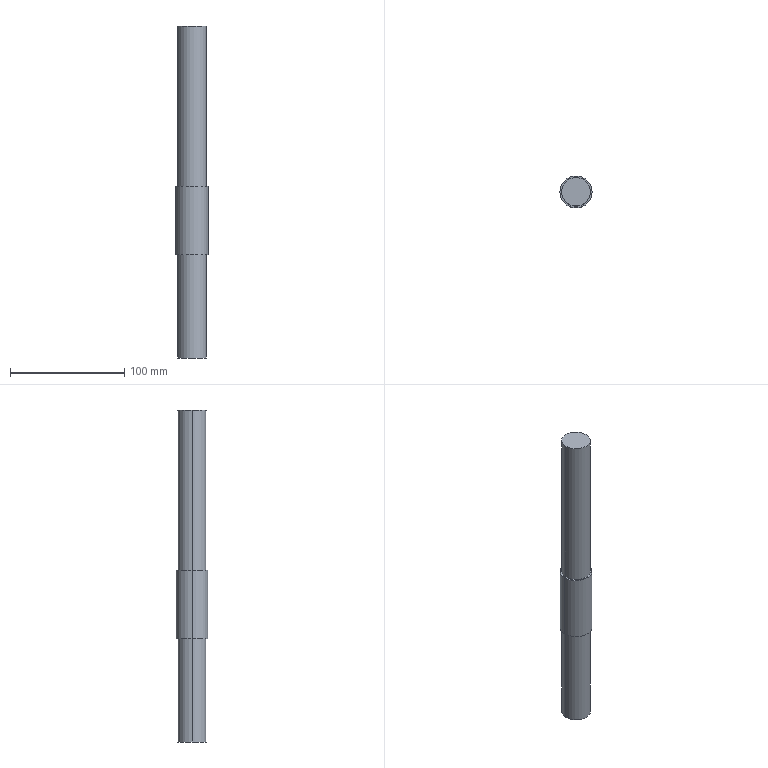Part | SolidWorks | features Revolution 1 | 1 solid | 10 faces | box 28 x 28 x 290 mm | volume 149846 mm3 | cylinder 6 | plane 4 | commonest cylinder face diameters 25 x4 28 x2
STEP:
#1=CARTESIAN_POINT('',(507.231,889.976,-240.893));
#2=VERTEX_POINT('',#1);
#3=CARTESIAN_POINT('',(535.231,889.976,-240.893));
#4=VERTEX_POINT('',#3);
#5=CARTESIAN_POINT('',(521.231,889.976,-240.893));
#6=DIRECTION('',(0.,0.,-1.));
#7=DIRECTION('',(-1.,0.,0.));
#8=AXIS2_PLACEMENT_3D('',#5,#6,#7);
#9=CIRCLE('',#8,14.);
#10=EDGE_CURVE('',#2,#4,#9,.T.);
#11=ORIENTED_EDGE('',*,*,#10,.T.);
#12=CARTESIAN_POINT('',(535.231,889.976,-300.893));
#13=VERTEX_POINT('',#12);
#14=CARTESIAN_POINT('',(535.231,889.976,-100.893));
#15=DIRECTION('',(0.,0.,-1.));
#16=VECTOR('',#15,1000.);
#17=LINE('',#14,#16);
#18=EDGE_CURVE('',#4,#13,#17,.T.);
#19=ORIENTED_EDGE('',*,*,#18,.T.);
#20=CARTESIAN_POINT('',(507.231,889.976,-300.893));
#21=VERTEX_POINT('',#20);
#22=CARTESIAN_POINT('',(521.231,889.976,-300.893));
#23=DIRECTION('',(0.,0.,-1.));
#24=DIRECTION('',(-1.,0.,0.));
#25=AXIS2_PLACEMENT_3D('',#22,#23,#24);
#26=CIRCLE('',#25,14.);
#27=EDGE_CURVE('',#21,#13,#26,.T.);
#28=ORIENTED_EDGE('',*,*,#27,.F.);
#29=CARTESIAN_POINT('',(507.231,889.976,-100.893));
#30=DIRECTION('',(0.,0.,-1.));
#31=VECTOR('',#30,1000.);
#32=LINE('',#29,#31);
#33=EDGE_CURVE('',#2,#21,#32,.T.);
#34=ORIENTED_EDGE('',*,*,#33,.F.);
#35=EDGE_LOOP('',(#11,#19,#28,#34));
#36=FACE_OUTER_BOUND('',#35,.T.);
#37=CARTESIAN_POINT('',(521.231,889.976,-100.893));
#38=DIRECTION('',(0.,0.,-1.));
#39=DIRECTION('',(-1.,0.,0.));
#40=AXIS2_PLACEMENT_3D('',#37,#38,#39);
#41=CYLINDRICAL_SURFACE('',#40,14.);
#42=ADVANCED_FACE('',(#36),#41,.T.);
#43=CARTESIAN_POINT('',(508.731,889.976,-300.893));
#44=VERTEX_POINT('',#43);
#45=CARTESIAN_POINT('',(533.731,889.976,-300.893));
#46=VERTEX_POINT('',#45);
#47=CARTESIAN_POINT('',(521.231,889.976,-300.893));
#48=DIRECTION('',(0.,0.,-1.));
#49=DIRECTION('',(-1.,0.,0.));
#50=AXIS2_PLACEMENT_3D('',#47,#48,#49);
#51=CIRCLE('',#50,12.5);
#52=EDGE_CURVE('',#44,#46,#51,.T.);
#53=ORIENTED_EDGE('',*,*,#52,.T.);
#54=CARTESIAN_POINT('',(533.731,889.976,-390.893));
#55=VERTEX_POINT('',#54);
#56=CARTESIAN_POINT('',(533.731,889.976,-100.893));
#57=DIRECTION('',(0.,0.,-1.));
#58=VECTOR('',#57,1000.);
#59=LINE('',#56,#58);
#60=EDGE_CURVE('',#46,#55,#59,.T.);
#61=ORIENTED_EDGE('',*,*,#60,.T.);
#62=CARTESIAN_POINT('',(508.731,889.976,-390.893));
#63=VERTEX_POINT('',#62);
#64=CARTESIAN_POINT('',(521.231,889.976,-390.893));
#65=DIRECTION('',(0.,0.,-1.));
#66=DIRECTION('',(-1.,0.,0.));
#67=AXIS2_PLACEMENT_3D('',#64,#65,#66);
#68=CIRCLE('',#67,12.5);
#69=EDGE_CURVE('',#63,#55,#68,.T.);
#70=ORIENTED_EDGE('',*,*,#69,.F.);
#71=CARTESIAN_POINT('',(508.731,889.976,-100.893));
#72=DIRECTION('',(0.,0.,-1.));
#73=VECTOR('',#72,1000.);
#74=LINE('',#71,#73);
#75=EDGE_CURVE('',#44,#63,#74,.T.);
#76=ORIENTED_EDGE('',*,*,#75,.F.);
#77=EDGE_LOOP('',(#53,#61,#70,#76));
#78=FACE_OUTER_BOUND('',#77,.T.);
#79=CARTESIAN_POINT('',(521.231,889.976,-100.893));
#80=DIRECTION('',(0.,0.,-1.));
#81=DIRECTION('',(-1.,0.,0.));
#82=AXIS2_PLACEMENT_3D('',#79,#80,#81);
#83=CYLINDRICAL_SURFACE('',#82,12.5);
#84=ADVANCED_FACE('',(#78),#83,.T.);
#85=CARTESIAN_POINT('',(508.731,889.976,-100.893));
#86=VERTEX_POINT('',#85);
#87=CARTESIAN_POINT('',(533.731,889.976,-100.893));
#88=VERTEX_POINT('',#87);
#89=CARTESIAN_POINT('',(521.231,889.976,-100.893));
#90=DIRECTION('',(0.,0.,-1.));
#91=DIRECTION('',(-1.,0.,0.));
#92=AXIS2_PLACEMENT_3D('',#89,#90,#91);
#93=CIRCLE('',#92,12.5);
#94=EDGE_CURVE('',#86,#88,#93,.T.);
#95=ORIENTED_EDGE('',*,*,#94,.T.);
#96=CARTESIAN_POINT('',(533.731,889.976,-240.893));
#97=VERTEX_POINT('',#96);
#98=CARTESIAN_POINT('',(533.731,889.976,-100.893));
#99=DIRECTION('',(0.,0.,-1.));
#100=VECTOR('',#99,1000.);
#101=LINE('',#98,#100);
#102=EDGE_CURVE('',#88,#97,#101,.T.);
#103=ORIENTED_EDGE('',*,*,#102,.T.);
#104=CARTESIAN_POINT('',(508.731,889.976,-240.893));
#105=VERTEX_POINT('',#104);
#106=CARTESIAN_POINT('',(521.231,889.976,-240.893));
#107=DIRECTION('',(0.,0.,-1.));
#108=DIRECTION('',(-1.,0.,0.));
#109=AXIS2_PLACEMENT_3D('',#106,#107,#108);
#110=CIRCLE('',#109,12.5);
#111=EDGE_CURVE('',#105,#97,#110,.T.);
#112=ORIENTED_EDGE('',*,*,#111,.F.);
#113=CARTESIAN_POINT('',(508.731,889.976,-100.893));
#114=DIRECTION('',(0.,0.,-1.));
#115=VECTOR('',#114,1000.);
#116=LINE('',#113,#115);
#117=EDGE_CURVE('',#86,#105,#116,.T.);
#118=ORIENTED_EDGE('',*,*,#117,.F.);
#119=EDGE_LOOP('',(#95,#103,#112,#118));
#120=FACE_OUTER_BOUND('',#119,.T.);
#121=CARTESIAN_POINT('',(521.231,889.976,-100.893));
#122=DIRECTION('',(0.,0.,-1.));
#123=DIRECTION('',(-1.,0.,0.));
#124=AXIS2_PLACEMENT_3D('',#121,#122,#123);
#125=CYLINDRICAL_SURFACE('',#124,12.5);
#126=ADVANCED_FACE('',(#120),#125,.T.);
#127=ORIENTED_EDGE('',*,*,#102,.F.);
#128=CARTESIAN_POINT('',(521.231,889.976,-100.893));
#129=DIRECTION('',(0.,0.,-1.));
#130=DIRECTION('',(-1.,0.,0.));
#131=AXIS2_PLACEMENT_3D('',#128,#129,#130);
#132=CIRCLE('',#131,12.5);
#133=EDGE_CURVE('',#88,#86,#132,.T.);
#134=ORIENTED_EDGE('',*,*,#133,.T.);
#135=ORIENTED_EDGE('',*,*,#117,.T.);
#136=CARTESIAN_POINT('',(521.231,889.976,-240.893));
#137=DIRECTION('',(0.,0.,-1.));
#138=DIRECTION('',(-1.,0.,0.));
#139=AXIS2_PLACEMENT_3D('',#136,#137,#138);
#140=CIRCLE('',#139,12.5);
#141=EDGE_CURVE('',#97,#105,#140,.T.);
#142=ORIENTED_EDGE('',*,*,#141,.F.);
#143=EDGE_LOOP('',(#127,#134,#135,#142));
#144=FACE_OUTER_BOUND('',#143,.T.);
#145=CARTESIAN_POINT('',(521.231,889.976,-100.893));
#146=DIRECTION('',(0.,0.,-1.));
#147=DIRECTION('',(-1.,0.,0.));
#148=AXIS2_PLACEMENT_3D('',#145,#146,#147);
#149=CYLINDRICAL_SURFACE('',#148,12.5);
#150=ADVANCED_FACE('',(#144),#149,.T.);
#151=ORIENTED_EDGE('',*,*,#94,.F.);
#152=ORIENTED_EDGE('',*,*,#133,.F.);
#153=EDGE_LOOP('',(#151,#152));
#154=FACE_OUTER_BOUND('',#153,.T.);
#155=CARTESIAN_POINT('',(533.731,889.976,-100.893));
#156=DIRECTION('',(0.,0.,1.));
#157=DIRECTION('',(1.,0.,0.));
#158=AXIS2_PLACEMENT_3D('',#155,#156,#157);
#159=PLANE('',#158);
#160=ADVANCED_FACE('',(#154),#159,.T.);
#161=ORIENTED_EDGE('',*,*,#69,.T.);
#162=CARTESIAN_POINT('',(521.231,889.976,-390.893));
#163=DIRECTION('',(0.,0.,-1.));
#164=DIRECTION('',(-1.,0.,0.));
#165=AXIS2_PLACEMENT_3D('',#162,#163,#164);
#166=CIRCLE('',#165,12.5);
#167=EDGE_CURVE('',#55,#63,#166,.T.);
#168=ORIENTED_EDGE('',*,*,#167,.T.);
#169=EDGE_LOOP('',(#161,#168));
#170=FACE_OUTER_BOUND('',#169,.T.);
#171=CARTESIAN_POINT('',(521.231,889.976,-390.893));
#172=DIRECTION('',(0.,0.,-1.));
#173=DIRECTION('',(-1.,0.,0.));
#174=AXIS2_PLACEMENT_3D('',#171,#172,#173);
#175=PLANE('',#174);
#176=ADVANCED_FACE('',(#170),#175,.T.);
#177=ORIENTED_EDGE('',*,*,#60,.F.);
#178=CARTESIAN_POINT('',(521.231,889.976,-300.893));
#179=DIRECTION('',(0.,0.,-1.));
#180=DIRECTION('',(-1.,0.,0.));
#181=AXIS2_PLACEMENT_3D('',#178,#179,#180);
#182=CIRCLE('',#181,12.5);
#183=EDGE_CURVE('',#46,#44,#182,.T.);
#184=ORIENTED_EDGE('',*,*,#183,.T.);
#185=ORIENTED_EDGE('',*,*,#75,.T.);
#186=ORIENTED_EDGE('',*,*,#167,.F.);
#187=EDGE_LOOP('',(#177,#184,#185,#186));
#188=FACE_OUTER_BOUND('',#187,.T.);
#189=CARTESIAN_POINT('',(521.231,889.976,-100.893));
#190=DIRECTION('',(0.,0.,-1.));
#191=DIRECTION('',(-1.,0.,0.));
#192=AXIS2_PLACEMENT_3D('',#189,#190,#191);
#193=CYLINDRICAL_SURFACE('',#192,12.5);
#194=ADVANCED_FACE('',(#188),#193,.T.);
#195=ORIENTED_EDGE('',*,*,#27,.T.);
#196=CARTESIAN_POINT('',(521.231,889.976,-300.893));
#197=DIRECTION('',(0.,0.,-1.));
#198=DIRECTION('',(-1.,0.,0.));
#199=AXIS2_PLACEMENT_3D('',#196,#197,#198);
#200=CIRCLE('',#199,14.);
#201=EDGE_CURVE('',#13,#21,#200,.T.);
#202=ORIENTED_EDGE('',*,*,#201,.T.);
#203=EDGE_LOOP('',(#195,#202));
#204=FACE_OUTER_BOUND('',#203,.T.);
#205=ORIENTED_EDGE('',*,*,#52,.F.);
#206=ORIENTED_EDGE('',*,*,#183,.F.);
#207=EDGE_LOOP('',(#205,#206));
#208=FACE_BOUND('',#207,.T.);
#209=CARTESIAN_POINT('',(533.731,889.976,-300.893));
#210=DIRECTION('',(0.,0.,-1.));
#211=DIRECTION('',(-1.,0.,0.));
#212=AXIS2_PLACEMENT_3D('',#209,#210,#211);
#213=PLANE('',#212);
#214=ADVANCED_FACE('',(#204,#208),#213,.T.);
#215=ORIENTED_EDGE('',*,*,#18,.F.);
#216=CARTESIAN_POINT('',(521.231,889.976,-240.893));
#217=DIRECTION('',(0.,0.,-1.));
#218=DIRECTION('',(-1.,0.,0.));
#219=AXIS2_PLACEMENT_3D('',#216,#217,#218);
#220=CIRCLE('',#219,14.);
#221=EDGE_CURVE('',#4,#2,#220,.T.);
#222=ORIENTED_EDGE('',*,*,#221,.T.);
#223=ORIENTED_EDGE('',*,*,#33,.T.);
#224=ORIENTED_EDGE('',*,*,#201,.F.);
#225=EDGE_LOOP('',(#215,#222,#223,#224));
#226=FACE_OUTER_BOUND('',#225,.T.);
#227=CARTESIAN_POINT('',(521.231,889.976,-100.893));
#228=DIRECTION('',(0.,0.,-1.));
#229=DIRECTION('',(-1.,0.,0.));
#230=AXIS2_PLACEMENT_3D('',#227,#228,#229);
#231=CYLINDRICAL_SURFACE('',#230,14.);
#232=ADVANCED_FACE('',(#226),#231,.T.);
#233=ORIENTED_EDGE('',*,*,#111,.T.);
#234=ORIENTED_EDGE('',*,*,#141,.T.);
#235=EDGE_LOOP('',(#233,#234));
#236=FACE_BOUND('',#235,.T.);
#237=ORIENTED_EDGE('',*,*,#10,.F.);
#238=ORIENTED_EDGE('',*,*,#221,.F.);
#239=EDGE_LOOP('',(#237,#238));
#240=FACE_OUTER_BOUND('',#239,.T.);
#241=CARTESIAN_POINT('',(535.231,889.976,-240.893));
#242=DIRECTION('',(0.,0.,1.));
#243=DIRECTION('',(1.,0.,0.));
#244=AXIS2_PLACEMENT_3D('',#241,#242,#243);
#245=PLANE('',#244);
#246=ADVANCED_FACE('',(#236,#240),#245,.T.);
#247=CLOSED_SHELL('',(#42,#84,#126,#150,#160,#176,#194,#214,#232,#246));
#248=MANIFOLD_SOLID_BREP('',#247);
#249=CARTESIAN_POINT('',(0.,0.,0.));
#250=DIRECTION('',(0.,0.,1.));
#251=DIRECTION('',(1.,0.,0.));
#252=AXIS2_PLACEMENT_3D('',#249,#250,#251);
#253=(LENGTH_UNIT()NAMED_UNIT(*)SI_UNIT(.MILLI.,.METRE.));
#254=UNCERTAINTY_MEASURE_WITH_UNIT(LENGTH_MEASURE(0.00001),#253,'','');
#255=(NAMED_UNIT(*)PLANE_ANGLE_UNIT()SI_UNIT($,.RADIAN.));
#256=(NAMED_UNIT(*)SI_UNIT($,.STERADIAN.)SOLID_ANGLE_UNIT());
#257=(GEOMETRIC_REPRESENTATION_CONTEXT(3)GLOBAL_UNCERTAINTY_ASSIGNED_CONTEXT((#254))GLOBAL_UNIT_ASSIGNED_CONTEXT((#253,#255,#256))REPRESENTATION_CONTEXT('',''));
#258=ADVANCED_BREP_SHAPE_REPRESENTATION('',(#248,#252),#257);